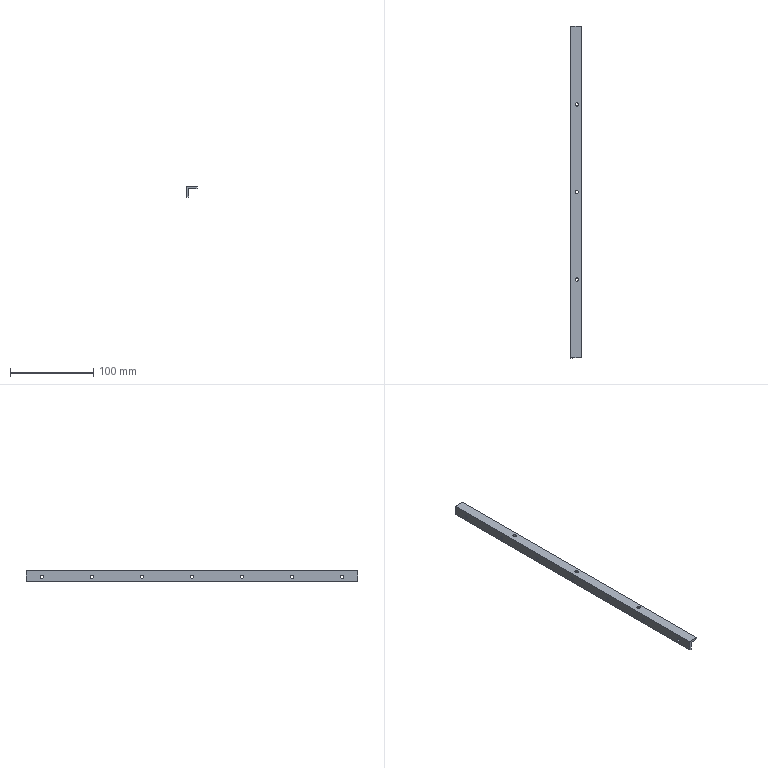Part | STEP file | 1-40.10 | 1 solid | 18 faces | box 12 x 398 x 12 mm | volume 17261 mm3 | cylinder 10 | plane 8 | commonest cylinder face diameters 4 x10